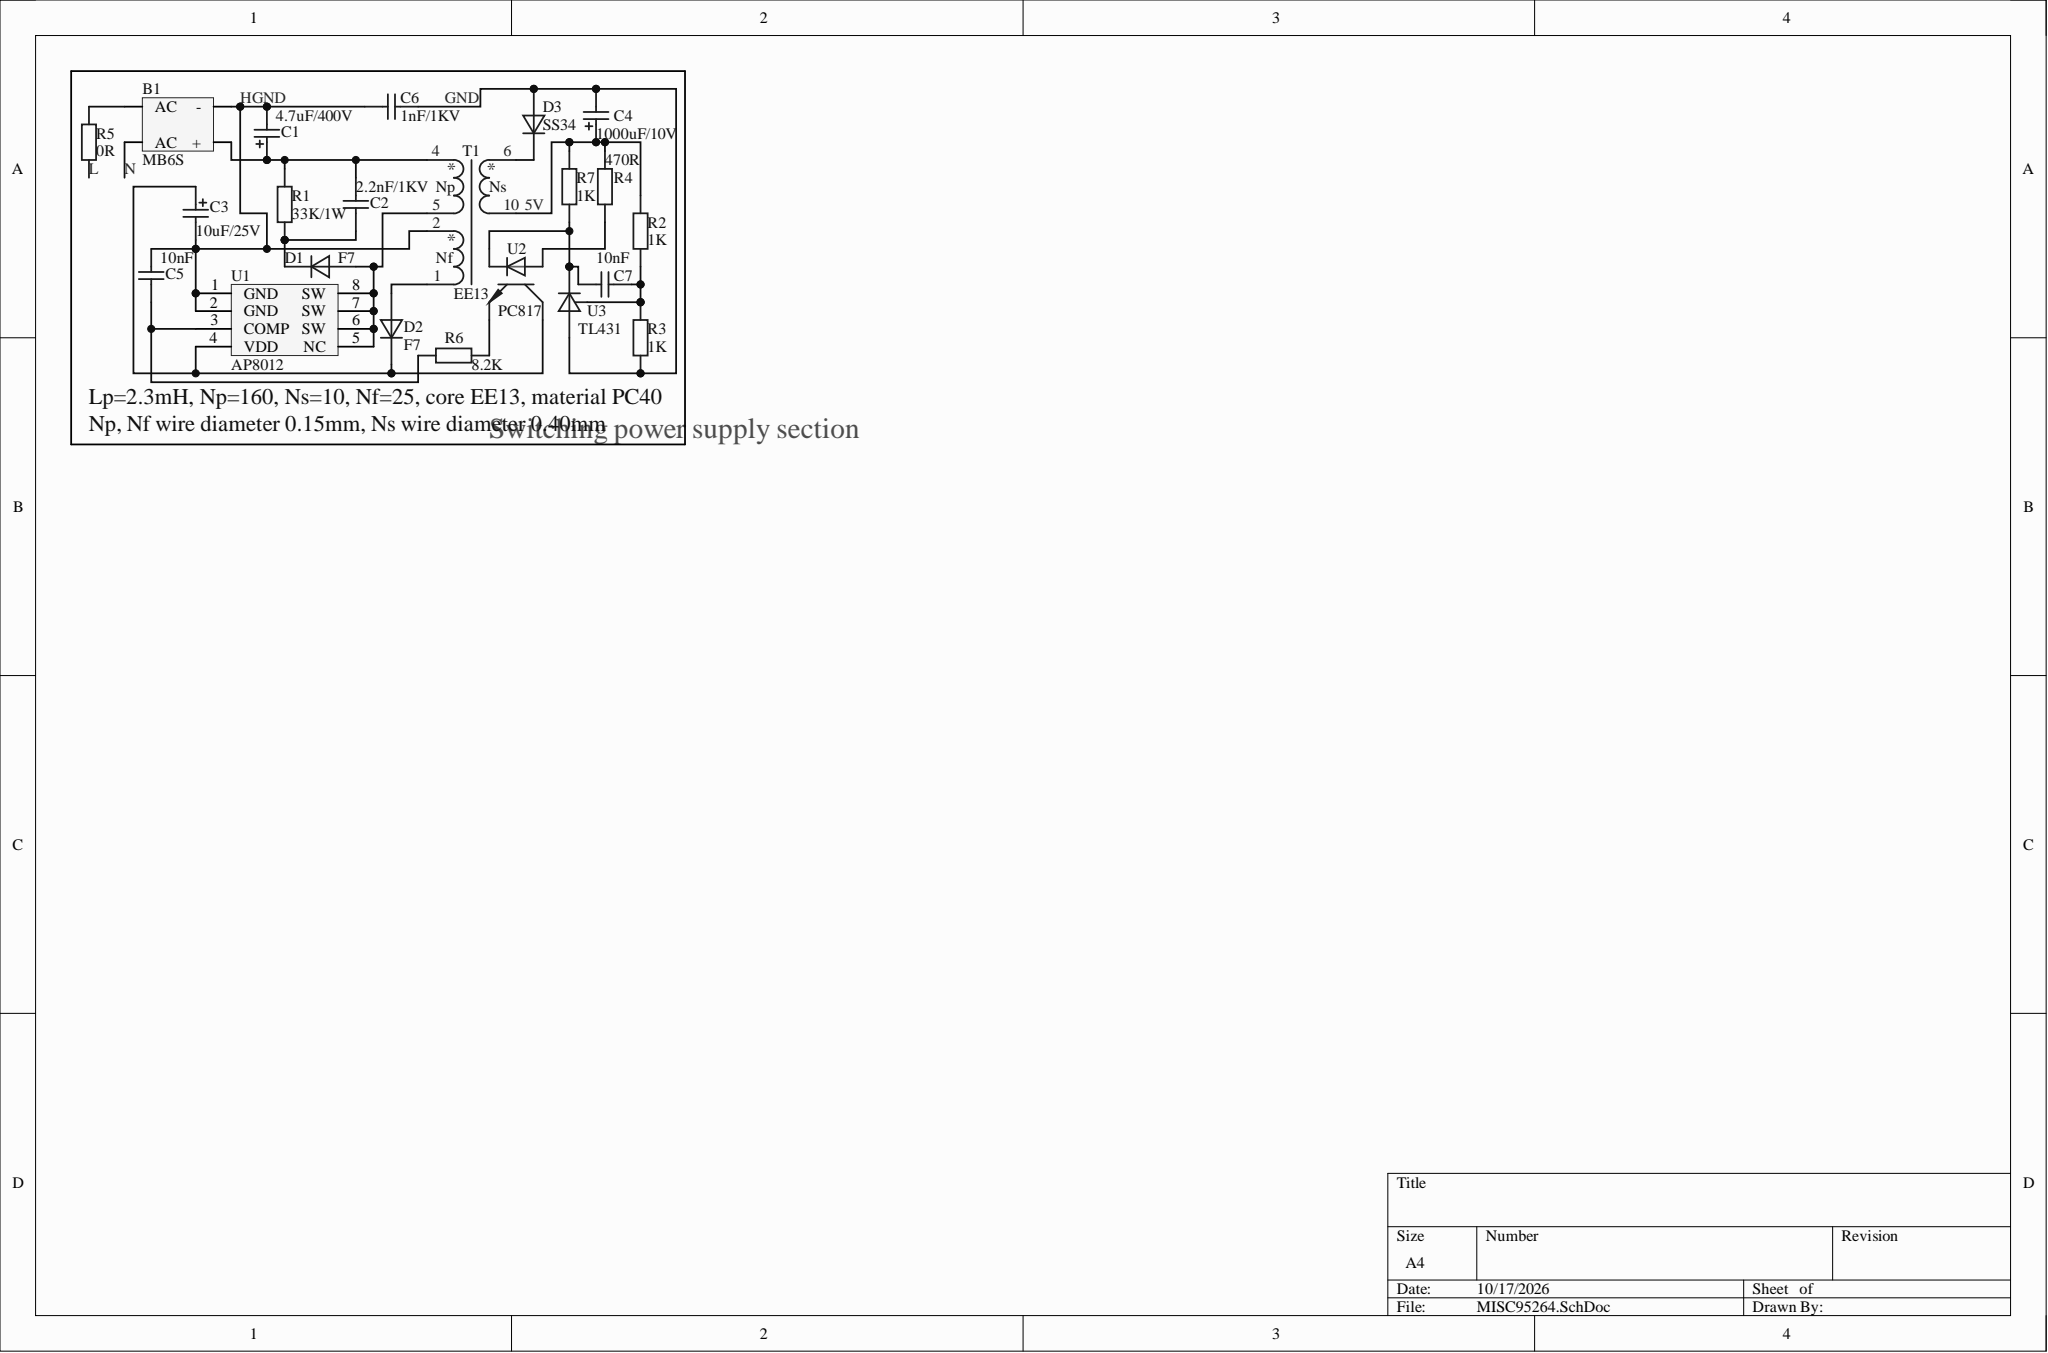Circuit board | Altium Designer | 22 parts | 15 nets
Bill of materials:
Comment,Description,Designator,Footprint,LibRef,Quantity
"MB6S","600V 0.8A Bridge Rectifiers","B1","SOP4","MB6S","1"
"4.7uF/400V","","C1","cap-8*14mm","Cap Pol","1"
"2.2nF/1KV","","C2","CAP_5mm","Cap","1"
"10uF/25V","","C3","cap-5*12mm","Cap Pol","1"
"1000uF/10V","","C4","cap-8*14mm","Cap Pol","1"
"10nF","","C5, C7","0805_Cap","Cap","2"
"1nF/1KV","","C6","CAP_5mm","Cap","1"
"F7","","D1, D2","SOD-123","Diode","2"
"SS34","","D3","DO_214AC/SMA","Diode","1"
"33K/1W","","R1","1W_Res_L","Res","1"
"1K","","R2, R3, R7","0805_Res","Res","3"
"470R","","R4","0805_Res","Res","1"
"0R","","R5","0805_Res","Res","1"
"8.2K","","R6","0805_Res","Res","1"
"EE13","","T1","EE13_5+5_L","Flyback transformer-1","1"
"AP8012","5W Flyback SMPS Controller","U1","DIP-8","AP8012","1"
"PC817","Device Specification For PhotoCoupler","U2","SOP4-PC817","PC817","1"
"TL431","Adjustable Precision Shunt Regulator","U3","TO-92","TL431","1"
Netlist (Protel format):
[
B1
SOP4
MB6S



]
[
C1
cap-8*14mm
4.7uF/400V



]
[
C2
CAP_5mm
2.2nF/1KV



]
[
C3
cap-5*12mm
10uF/25V



]
[
C4
cap-8*14mm
1000uF/10V



]
[
C5
0805_Cap
10nF



]
[
C6
CAP_5mm
1nF/1KV



]
[
C7
0805_Cap
10nF



]
[
D1
SOD-123
F7



]
[
D2
SOD-123
F7



]
[
D3
DO_214AC/SMA
SS34



]
[
R1
1W_Res_L
33K/1W



]
[
R2
0805_Res
1K



]
[
R3
0805_Res
1K



]
[
R4
0805_Res
470R



]
[
R5
0805_Res
0R



]
[
R6
0805_Res
8.2K



]
[
R7
0805_Res
1K



]
[
T1
EE13_5+5_L
EE13



]
[
U1
DIP-8
AP8012



]
[
U2
SOP4-PC817
PC817



]
[
U3
TO-92
TL431



]
(
NetR6_2
R6-2
U2-3
)
(
NetR4_1
R4-1
U2-1
)
(
NetD3_2
D3-2
T1-6
)
(
NetD2_1
D2-1
T1-1
)
(
NetD1_1
D1-1
T1-5
U1-5
U1-6
U1-7
U1-8
)
(
NetC7_2
C7-2
R2-1
R3-2
U3-1
)
(
NetC7_1
C7-1
R7-1
U2-2
U3-3
)
(
NetC5_1
C5-1
R6-1
U1-3
)
(
NetC3_1
C3-1
D2-2
U1-4
U2-4
)
(
NetC2_1
C2-1
D1-2
R1-2
)
(
NetB1_3
B1-3
C1-1
C2-2
R1-1
T1-4
)
(
NetB1_1
B1-1
R5-2
)
(
HGND
B1-4
C1-2
C3-2
C5-2
C6-2
T1-2
U1-1
U1-2
)
(
GND
C4-2
C6-1
D3-1
R3-1
U3-2
)
(
5V
C4-1
R2-2
R4-2
R7-2
T1-10
)